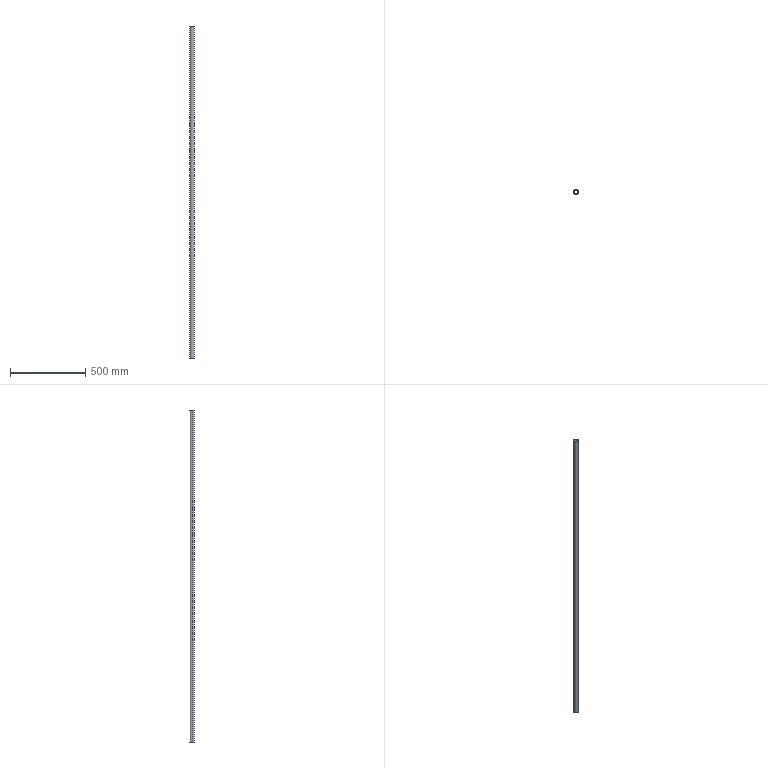Part | SolidWorks | features Extrusion 1 | 1 solid | 6 faces | box 32 x 32 x 2210 mm | volume 416575 mm3 | cylinder 4 | plane 2 | commonest cylinder face diameters 28 x2 32 x2
STEP:
#1=CARTESIAN_POINT('',(-14.,0.,1105.));
#2=VERTEX_POINT('',#1);
#3=CARTESIAN_POINT('',(14.,0.,1105.));
#4=VERTEX_POINT('',#3);
#5=CARTESIAN_POINT('',(0.,0.,1105.));
#6=DIRECTION('',(0.,0.,1.));
#7=DIRECTION('',(1.,0.,0.));
#8=AXIS2_PLACEMENT_3D('',#5,#6,#7);
#9=CIRCLE('',#8,14.);
#10=EDGE_CURVE('',#2,#4,#9,.T.);
#11=ORIENTED_EDGE('',*,*,#10,.T.);
#12=CARTESIAN_POINT('',(14.,0.,-1105.));
#13=VERTEX_POINT('',#12);
#14=CARTESIAN_POINT('',(14.,0.,1105.));
#15=DIRECTION('',(0.,0.,-1.));
#16=VECTOR('',#15,1000.);
#17=LINE('',#14,#16);
#18=EDGE_CURVE('',#4,#13,#17,.T.);
#19=ORIENTED_EDGE('',*,*,#18,.T.);
#20=CARTESIAN_POINT('',(-14.,0.,-1105.));
#21=VERTEX_POINT('',#20);
#22=CARTESIAN_POINT('',(0.,0.,-1105.));
#23=DIRECTION('',(0.,0.,1.));
#24=DIRECTION('',(1.,0.,0.));
#25=AXIS2_PLACEMENT_3D('',#22,#23,#24);
#26=CIRCLE('',#25,14.);
#27=EDGE_CURVE('',#21,#13,#26,.T.);
#28=ORIENTED_EDGE('',*,*,#27,.F.);
#29=CARTESIAN_POINT('',(-14.,0.,1105.));
#30=DIRECTION('',(0.,0.,-1.));
#31=VECTOR('',#30,1000.);
#32=LINE('',#29,#31);
#33=EDGE_CURVE('',#2,#21,#32,.T.);
#34=ORIENTED_EDGE('',*,*,#33,.F.);
#35=EDGE_LOOP('',(#11,#19,#28,#34));
#36=FACE_OUTER_BOUND('',#35,.T.);
#37=CARTESIAN_POINT('',(0.,0.,1105.));
#38=DIRECTION('',(0.,0.,-1.));
#39=DIRECTION('',(-1.,0.,0.));
#40=AXIS2_PLACEMENT_3D('',#37,#38,#39);
#41=CYLINDRICAL_SURFACE('',#40,14.);
#42=ADVANCED_FACE('',(#36),#41,.F.);
#43=CARTESIAN_POINT('',(16.,0.,1105.));
#44=VERTEX_POINT('',#43);
#45=CARTESIAN_POINT('',(-16.,0.,1105.));
#46=VERTEX_POINT('',#45);
#47=CARTESIAN_POINT('',(0.,0.,1105.));
#48=DIRECTION('',(0.,0.,1.));
#49=DIRECTION('',(1.,0.,0.));
#50=AXIS2_PLACEMENT_3D('',#47,#48,#49);
#51=CIRCLE('',#50,16.);
#52=EDGE_CURVE('',#44,#46,#51,.T.);
#53=ORIENTED_EDGE('',*,*,#52,.F.);
#54=CARTESIAN_POINT('',(16.,0.,-1105.));
#55=VERTEX_POINT('',#54);
#56=CARTESIAN_POINT('',(16.,0.,1105.));
#57=DIRECTION('',(0.,0.,-1.));
#58=VECTOR('',#57,1000.);
#59=LINE('',#56,#58);
#60=EDGE_CURVE('',#44,#55,#59,.T.);
#61=ORIENTED_EDGE('',*,*,#60,.T.);
#62=CARTESIAN_POINT('',(-16.,0.,-1105.));
#63=VERTEX_POINT('',#62);
#64=CARTESIAN_POINT('',(0.,0.,-1105.));
#65=DIRECTION('',(0.,0.,1.));
#66=DIRECTION('',(1.,0.,0.));
#67=AXIS2_PLACEMENT_3D('',#64,#65,#66);
#68=CIRCLE('',#67,16.);
#69=EDGE_CURVE('',#55,#63,#68,.T.);
#70=ORIENTED_EDGE('',*,*,#69,.T.);
#71=CARTESIAN_POINT('',(-16.,0.,1105.));
#72=DIRECTION('',(0.,0.,-1.));
#73=VECTOR('',#72,1000.);
#74=LINE('',#71,#73);
#75=EDGE_CURVE('',#46,#63,#74,.T.);
#76=ORIENTED_EDGE('',*,*,#75,.F.);
#77=EDGE_LOOP('',(#53,#61,#70,#76));
#78=FACE_OUTER_BOUND('',#77,.T.);
#79=CARTESIAN_POINT('',(0.,0.,1105.));
#80=DIRECTION('',(0.,0.,-1.));
#81=DIRECTION('',(-1.,0.,0.));
#82=AXIS2_PLACEMENT_3D('',#79,#80,#81);
#83=CYLINDRICAL_SURFACE('',#82,16.);
#84=ADVANCED_FACE('',(#78),#83,.T.);
#85=CARTESIAN_POINT('',(0.,0.,1105.));
#86=DIRECTION('',(0.,0.,1.));
#87=DIRECTION('',(1.,0.,0.));
#88=AXIS2_PLACEMENT_3D('',#85,#86,#87);
#89=CIRCLE('',#88,16.);
#90=EDGE_CURVE('',#46,#44,#89,.T.);
#91=ORIENTED_EDGE('',*,*,#90,.T.);
#92=ORIENTED_EDGE('',*,*,#52,.T.);
#93=EDGE_LOOP('',(#91,#92));
#94=FACE_OUTER_BOUND('',#93,.T.);
#95=ORIENTED_EDGE('',*,*,#10,.F.);
#96=CARTESIAN_POINT('',(0.,0.,1105.));
#97=DIRECTION('',(0.,0.,1.));
#98=DIRECTION('',(1.,0.,0.));
#99=AXIS2_PLACEMENT_3D('',#96,#97,#98);
#100=CIRCLE('',#99,14.);
#101=EDGE_CURVE('',#4,#2,#100,.T.);
#102=ORIENTED_EDGE('',*,*,#101,.F.);
#103=EDGE_LOOP('',(#95,#102));
#104=FACE_BOUND('',#103,.T.);
#105=CARTESIAN_POINT('',(0.,0.,1105.));
#106=DIRECTION('',(0.,0.,1.));
#107=DIRECTION('',(1.,0.,0.));
#108=AXIS2_PLACEMENT_3D('',#105,#106,#107);
#109=PLANE('',#108);
#110=ADVANCED_FACE('',(#94,#104),#109,.T.);
#111=CARTESIAN_POINT('',(0.,0.,-1105.));
#112=DIRECTION('',(0.,0.,1.));
#113=DIRECTION('',(1.,0.,0.));
#114=AXIS2_PLACEMENT_3D('',#111,#112,#113);
#115=CIRCLE('',#114,16.);
#116=EDGE_CURVE('',#63,#55,#115,.T.);
#117=ORIENTED_EDGE('',*,*,#116,.F.);
#118=ORIENTED_EDGE('',*,*,#69,.F.);
#119=EDGE_LOOP('',(#117,#118));
#120=FACE_OUTER_BOUND('',#119,.T.);
#121=ORIENTED_EDGE('',*,*,#27,.T.);
#122=CARTESIAN_POINT('',(0.,0.,-1105.));
#123=DIRECTION('',(0.,0.,1.));
#124=DIRECTION('',(1.,0.,0.));
#125=AXIS2_PLACEMENT_3D('',#122,#123,#124);
#126=CIRCLE('',#125,14.);
#127=EDGE_CURVE('',#13,#21,#126,.T.);
#128=ORIENTED_EDGE('',*,*,#127,.T.);
#129=EDGE_LOOP('',(#121,#128));
#130=FACE_BOUND('',#129,.T.);
#131=CARTESIAN_POINT('',(0.,0.,-1105.));
#132=DIRECTION('',(0.,0.,1.));
#133=DIRECTION('',(1.,0.,0.));
#134=AXIS2_PLACEMENT_3D('',#131,#132,#133);
#135=PLANE('',#134);
#136=ADVANCED_FACE('',(#120,#130),#135,.F.);
#137=ORIENTED_EDGE('',*,*,#60,.F.);
#138=ORIENTED_EDGE('',*,*,#90,.F.);
#139=ORIENTED_EDGE('',*,*,#75,.T.);
#140=ORIENTED_EDGE('',*,*,#116,.T.);
#141=EDGE_LOOP('',(#137,#138,#139,#140));
#142=FACE_OUTER_BOUND('',#141,.T.);
#143=CARTESIAN_POINT('',(0.,0.,1105.));
#144=DIRECTION('',(0.,0.,-1.));
#145=DIRECTION('',(-1.,0.,0.));
#146=AXIS2_PLACEMENT_3D('',#143,#144,#145);
#147=CYLINDRICAL_SURFACE('',#146,16.);
#148=ADVANCED_FACE('',(#142),#147,.T.);
#149=ORIENTED_EDGE('',*,*,#18,.F.);
#150=ORIENTED_EDGE('',*,*,#101,.T.);
#151=ORIENTED_EDGE('',*,*,#33,.T.);
#152=ORIENTED_EDGE('',*,*,#127,.F.);
#153=EDGE_LOOP('',(#149,#150,#151,#152));
#154=FACE_OUTER_BOUND('',#153,.T.);
#155=CARTESIAN_POINT('',(0.,0.,1105.));
#156=DIRECTION('',(0.,0.,-1.));
#157=DIRECTION('',(-1.,0.,0.));
#158=AXIS2_PLACEMENT_3D('',#155,#156,#157);
#159=CYLINDRICAL_SURFACE('',#158,14.);
#160=ADVANCED_FACE('',(#154),#159,.F.);
#161=CLOSED_SHELL('',(#42,#84,#110,#136,#148,#160));
#162=MANIFOLD_SOLID_BREP('',#161);
#163=CARTESIAN_POINT('',(0.,0.,0.));
#164=DIRECTION('',(0.,0.,1.));
#165=DIRECTION('',(1.,0.,0.));
#166=AXIS2_PLACEMENT_3D('',#163,#164,#165);
#167=(LENGTH_UNIT()NAMED_UNIT(*)SI_UNIT(.MILLI.,.METRE.));
#168=UNCERTAINTY_MEASURE_WITH_UNIT(LENGTH_MEASURE(0.00001),#167,'','');
#169=(NAMED_UNIT(*)PLANE_ANGLE_UNIT()SI_UNIT($,.RADIAN.));
#170=(NAMED_UNIT(*)SI_UNIT($,.STERADIAN.)SOLID_ANGLE_UNIT());
#171=(GEOMETRIC_REPRESENTATION_CONTEXT(3)GLOBAL_UNCERTAINTY_ASSIGNED_CONTEXT((#168))GLOBAL_UNIT_ASSIGNED_CONTEXT((#167,#169,#170))REPRESENTATION_CONTEXT('',''));
#172=ADVANCED_BREP_SHAPE_REPRESENTATION('',(#162,#166),#171);